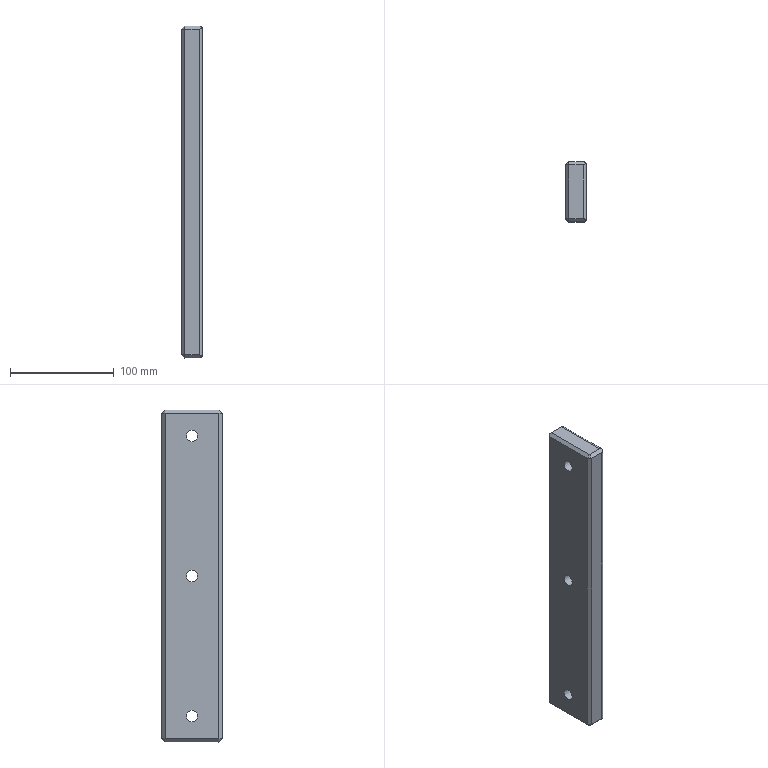Part | STEP file | lll_id1718_x_t | 1 solid | 31 faces | box 20 x 58 x 320 mm | volume 355635 mm3 | plane 21 | cylinder 10 | commonest cylinder face diameters 6 x4 11 x3 17 x3
STEP:
#1=CARTESIAN_POINT('',(2151.435,-651.5,-282.5));
#2=VERTEX_POINT('',#1);
#3=CARTESIAN_POINT('',(2151.435,-651.5,31.5));
#4=VERTEX_POINT('',#3);
#5=CARTESIAN_POINT('',(2151.435,-651.5,-55.5));
#6=DIRECTION('',(0.,-0.000000092,1.));
#7=VECTOR('',#6,1.);
#8=LINE('',#5,#7);
#9=EDGE_CURVE('',#2,#4,#8,.T.);
#10=ORIENTED_EDGE('',*,*,#9,.T.);
#11=CARTESIAN_POINT('',(2151.435,-599.5,31.5));
#12=VERTEX_POINT('',#11);
#13=CARTESIAN_POINT('',(2151.435,-644.5,31.5));
#14=DIRECTION('',(0.,1.,0.000000092));
#15=VECTOR('',#14,1.);
#16=LINE('',#13,#15);
#17=EDGE_CURVE('',#4,#12,#16,.T.);
#18=ORIENTED_EDGE('',*,*,#17,.T.);
#19=CARTESIAN_POINT('',(2151.435,-599.5,-282.5));
#20=VERTEX_POINT('',#19);
#21=CARTESIAN_POINT('',(2151.435,-599.5,69.5));
#22=DIRECTION('',(0.,0.000000092,-1.));
#23=VECTOR('',#22,1.);
#24=LINE('',#21,#23);
#25=EDGE_CURVE('',#12,#20,#24,.T.);
#26=ORIENTED_EDGE('',*,*,#25,.T.);
#27=CARTESIAN_POINT('',(2151.435,-596.5,-282.5));
#28=DIRECTION('',(0.,-1.,-0.000000092));
#29=VECTOR('',#28,1.);
#30=LINE('',#27,#29);
#31=EDGE_CURVE('',#20,#2,#30,.T.);
#32=ORIENTED_EDGE('',*,*,#31,.T.);
#33=EDGE_LOOP('',(#10,#18,#26,#32));
#34=FACE_BOUND('',#33,.T.);
#35=CARTESIAN_POINT('',(2151.435,-625.5,-266.));
#36=VERTEX_POINT('',#35);
#37=CARTESIAN_POINT('',(2151.435,-625.5,-260.5));
#38=DIRECTION('',(1.,0.,0.));
#39=DIRECTION('',(0.,0.,-1.));
#40=AXIS2_PLACEMENT_3D('',#37,#38,#39);
#41=CIRCLE('',#40,5.5);
#42=EDGE_CURVE('',#36,#36,#41,.T.);
#43=ORIENTED_EDGE('',*,*,#42,.T.);
#44=EDGE_LOOP('',(#43));
#45=FACE_BOUND('',#44,.T.);
#46=CARTESIAN_POINT('',(2151.435,-625.5,15.));
#47=VERTEX_POINT('',#46);
#48=CARTESIAN_POINT('',(2151.435,-625.5,9.5));
#49=DIRECTION('',(-1.,0.,0.));
#50=DIRECTION('',(0.,-0.000000184,1.));
#51=AXIS2_PLACEMENT_3D('',#48,#49,#50);
#52=CIRCLE('',#51,5.5);
#53=EDGE_CURVE('',#47,#47,#52,.T.);
#54=ORIENTED_EDGE('',*,*,#53,.F.);
#55=EDGE_LOOP('',(#54));
#56=FACE_BOUND('',#55,.T.);
#57=CARTESIAN_POINT('',(2151.435,-625.5,-131.));
#58=VERTEX_POINT('',#57);
#59=CARTESIAN_POINT('',(2151.435,-625.5,-125.5));
#60=DIRECTION('',(1.,0.,0.));
#61=DIRECTION('',(0.,0.,-1.));
#62=AXIS2_PLACEMENT_3D('',#59,#60,#61);
#63=CIRCLE('',#62,5.5);
#64=EDGE_CURVE('',#58,#58,#63,.T.);
#65=ORIENTED_EDGE('',*,*,#64,.T.);
#66=EDGE_LOOP('',(#65));
#67=FACE_BOUND('',#66,.T.);
#68=CARTESIAN_POINT('',(2151.435,-596.5,-55.5));
#69=DIRECTION('',(1.,0.,0.));
#70=DIRECTION('',(0.,-0.000000092,1.));
#71=AXIS2_PLACEMENT_3D('',#68,#69,#70);
#72=PLANE('',#71);
#73=ADVANCED_FACE('',(#34,#45,#56,#67),#72,.F.);
#74=CARTESIAN_POINT('',(2171.435,-625.5,-117.));
#75=VERTEX_POINT('',#74);
#76=CARTESIAN_POINT('',(2171.435,-625.5,-125.5));
#77=DIRECTION('',(-1.,0.,0.));
#78=DIRECTION('',(0.,0.,1.));
#79=AXIS2_PLACEMENT_3D('',#76,#77,#78);
#80=CIRCLE('',#79,8.5);
#81=EDGE_CURVE('',#75,#75,#80,.T.);
#82=ORIENTED_EDGE('',*,*,#81,.T.);
#83=EDGE_LOOP('',(#82));
#84=FACE_BOUND('',#83,.T.);
#85=CARTESIAN_POINT('',(2171.435,-599.5,31.5));
#86=VERTEX_POINT('',#85);
#87=CARTESIAN_POINT('',(2171.435,-599.5,-282.5));
#88=VERTEX_POINT('',#87);
#89=CARTESIAN_POINT('',(2171.435,-599.5,-55.5));
#90=DIRECTION('',(0.,0.000000092,-1.));
#91=VECTOR('',#90,1.);
#92=LINE('',#89,#91);
#93=EDGE_CURVE('',#86,#88,#92,.T.);
#94=ORIENTED_EDGE('',*,*,#93,.F.);
#95=CARTESIAN_POINT('',(2171.435,-651.5,31.5));
#96=VERTEX_POINT('',#95);
#97=CARTESIAN_POINT('',(2171.435,-644.5,31.5));
#98=DIRECTION('',(0.,-1.,-0.000000092));
#99=VECTOR('',#98,1.);
#100=LINE('',#97,#99);
#101=EDGE_CURVE('',#86,#96,#100,.T.);
#102=ORIENTED_EDGE('',*,*,#101,.T.);
#103=CARTESIAN_POINT('',(2171.435,-651.5,-282.5));
#104=VERTEX_POINT('',#103);
#105=CARTESIAN_POINT('',(2171.435,-651.5,-55.5));
#106=DIRECTION('',(0.,-0.000000092,1.));
#107=VECTOR('',#106,1.);
#108=LINE('',#105,#107);
#109=EDGE_CURVE('',#104,#96,#108,.T.);
#110=ORIENTED_EDGE('',*,*,#109,.F.);
#111=CARTESIAN_POINT('',(2171.435,-596.5,-282.5));
#112=DIRECTION('',(0.,-1.,-0.000000092));
#113=VECTOR('',#112,1.);
#114=LINE('',#111,#113);
#115=EDGE_CURVE('',#88,#104,#114,.T.);
#116=ORIENTED_EDGE('',*,*,#115,.F.);
#117=EDGE_LOOP('',(#94,#102,#110,#116));
#118=FACE_BOUND('',#117,.T.);
#119=CARTESIAN_POINT('',(2171.435,-625.5,-269.));
#120=VERTEX_POINT('',#119);
#121=CARTESIAN_POINT('',(2171.435,-625.5,-260.5));
#122=DIRECTION('',(-1.,0.,0.));
#123=DIRECTION('',(0.,0.,-1.));
#124=AXIS2_PLACEMENT_3D('',#121,#122,#123);
#125=CIRCLE('',#124,8.5);
#126=EDGE_CURVE('',#120,#120,#125,.T.);
#127=ORIENTED_EDGE('',*,*,#126,.T.);
#128=EDGE_LOOP('',(#127));
#129=FACE_BOUND('',#128,.T.);
#130=CARTESIAN_POINT('',(2171.435,-625.5,18.));
#131=VERTEX_POINT('',#130);
#132=CARTESIAN_POINT('',(2171.435,-625.5,9.5));
#133=DIRECTION('',(1.,0.,0.));
#134=DIRECTION('',(0.,-0.000000184,1.));
#135=AXIS2_PLACEMENT_3D('',#132,#133,#134);
#136=CIRCLE('',#135,8.5);
#137=EDGE_CURVE('',#131,#131,#136,.T.);
#138=ORIENTED_EDGE('',*,*,#137,.F.);
#139=EDGE_LOOP('',(#138));
#140=FACE_BOUND('',#139,.T.);
#141=CARTESIAN_POINT('',(2171.435,-596.5,-55.5));
#142=DIRECTION('',(1.,0.,0.));
#143=DIRECTION('',(0.,-0.000000092,1.));
#144=AXIS2_PLACEMENT_3D('',#141,#142,#143);
#145=PLANE('',#144);
#146=ADVANCED_FACE('',(#84,#118,#129,#140),#145,.T.);
#147=CARTESIAN_POINT('',(2154.435,-596.5,-282.5));
#148=VERTEX_POINT('',#147);
#149=CARTESIAN_POINT('',(2154.435,-596.5,31.5));
#150=VERTEX_POINT('',#149);
#151=CARTESIAN_POINT('',(2154.435,-596.5,69.5));
#152=DIRECTION('',(0.,-0.000000092,1.));
#153=VECTOR('',#152,1.);
#154=LINE('',#151,#153);
#155=EDGE_CURVE('',#148,#150,#154,.T.);
#156=ORIENTED_EDGE('',*,*,#155,.T.);
#157=CARTESIAN_POINT('',(2168.435,-596.5,31.5));
#158=VERTEX_POINT('',#157);
#159=CARTESIAN_POINT('',(2171.435,-596.5,31.5));
#160=DIRECTION('',(1.,0.,0.));
#161=VECTOR('',#160,1.);
#162=LINE('',#159,#161);
#163=EDGE_CURVE('',#150,#158,#162,.T.);
#164=ORIENTED_EDGE('',*,*,#163,.T.);
#165=CARTESIAN_POINT('',(2168.435,-596.5,-282.5));
#166=VERTEX_POINT('',#165);
#167=CARTESIAN_POINT('',(2168.435,-596.5,-55.5));
#168=DIRECTION('',(0.,-0.000000092,1.));
#169=VECTOR('',#168,1.);
#170=LINE('',#167,#169);
#171=EDGE_CURVE('',#166,#158,#170,.T.);
#172=ORIENTED_EDGE('',*,*,#171,.F.);
#173=CARTESIAN_POINT('',(2171.435,-596.5,-282.5));
#174=DIRECTION('',(-1.,0.,0.));
#175=VECTOR('',#174,1.);
#176=LINE('',#173,#175);
#177=EDGE_CURVE('',#166,#148,#176,.T.);
#178=ORIENTED_EDGE('',*,*,#177,.T.);
#179=EDGE_LOOP('',(#156,#164,#172,#178));
#180=FACE_OUTER_BOUND('',#179,.T.);
#181=CARTESIAN_POINT('',(2171.435,-596.5,69.5));
#182=DIRECTION('',(0.,-1.,-0.000000092));
#183=DIRECTION('',(0.,0.000000092,-1.));
#184=AXIS2_PLACEMENT_3D('',#181,#182,#183);
#185=PLANE('',#184);
#186=ADVANCED_FACE('',(#180),#185,.F.);
#187=CARTESIAN_POINT('',(2168.435,-654.5,31.5));
#188=VERTEX_POINT('',#187);
#189=CARTESIAN_POINT('',(2168.435,-654.5,-282.5));
#190=VERTEX_POINT('',#189);
#191=CARTESIAN_POINT('',(2168.435,-654.5,69.5));
#192=DIRECTION('',(0.,0.000000092,-1.));
#193=VECTOR('',#192,1.);
#194=LINE('',#191,#193);
#195=EDGE_CURVE('',#188,#190,#194,.T.);
#196=ORIENTED_EDGE('',*,*,#195,.F.);
#197=CARTESIAN_POINT('',(2154.435,-654.5,31.5));
#198=VERTEX_POINT('',#197);
#199=CARTESIAN_POINT('',(2171.435,-654.5,31.5));
#200=DIRECTION('',(-1.,0.,0.));
#201=VECTOR('',#200,1.);
#202=LINE('',#199,#201);
#203=EDGE_CURVE('',#188,#198,#202,.T.);
#204=ORIENTED_EDGE('',*,*,#203,.T.);
#205=CARTESIAN_POINT('',(2154.435,-654.5,-282.5));
#206=VERTEX_POINT('',#205);
#207=CARTESIAN_POINT('',(2154.435,-654.5,-55.5));
#208=DIRECTION('',(0.,0.000000092,-1.));
#209=VECTOR('',#208,1.);
#210=LINE('',#207,#209);
#211=EDGE_CURVE('',#198,#206,#210,.T.);
#212=ORIENTED_EDGE('',*,*,#211,.T.);
#213=CARTESIAN_POINT('',(2171.435,-654.5,-282.5));
#214=DIRECTION('',(1.,0.,0.));
#215=VECTOR('',#214,1.);
#216=LINE('',#213,#215);
#217=EDGE_CURVE('',#206,#190,#216,.T.);
#218=ORIENTED_EDGE('',*,*,#217,.T.);
#219=EDGE_LOOP('',(#196,#204,#212,#218));
#220=FACE_OUTER_BOUND('',#219,.T.);
#221=CARTESIAN_POINT('',(2171.435,-654.5,-55.5));
#222=DIRECTION('',(0.,1.,0.000000092));
#223=DIRECTION('',(0.,-0.000000092,1.));
#224=AXIS2_PLACEMENT_3D('',#221,#222,#223);
#225=PLANE('',#224);
#226=ADVANCED_FACE('',(#220),#225,.F.);
#227=ORIENTED_EDGE('',*,*,#171,.T.);
#228=CARTESIAN_POINT('',(2171.033,-598.,33.));
#229=VERTEX_POINT('',#228);
#230=CARTESIAN_POINT('',(2168.435,-599.5,34.5));
#231=DIRECTION('',(0.,-0.7071,-0.7071));
#232=DIRECTION('',(0.,-0.7071,0.7071));
#233=AXIS2_PLACEMENT_3D('',#230,#231,#232);
#234=ELLIPSE('',#233,4.243,3.);
#235=EDGE_CURVE('',#158,#229,#234,.T.);
#236=ORIENTED_EDGE('',*,*,#235,.T.);
#237=CARTESIAN_POINT('',(2168.435,-599.5,31.5));
#238=DIRECTION('',(0.,0.7071,-0.7071));
#239=DIRECTION('',(0.,0.7071,0.7071));
#240=AXIS2_PLACEMENT_3D('',#237,#238,#239);
#241=ELLIPSE('',#240,4.243,3.);
#242=EDGE_CURVE('',#229,#86,#241,.T.);
#243=ORIENTED_EDGE('',*,*,#242,.T.);
#244=ORIENTED_EDGE('',*,*,#93,.T.);
#245=CARTESIAN_POINT('',(2171.033,-598.,-284.));
#246=VERTEX_POINT('',#245);
#247=CARTESIAN_POINT('',(2168.435,-599.5,-282.5));
#248=DIRECTION('',(0.,-0.7071,-0.7071));
#249=DIRECTION('',(0.,0.7071,-0.7071));
#250=AXIS2_PLACEMENT_3D('',#247,#248,#249);
#251=ELLIPSE('',#250,4.243,3.);
#252=EDGE_CURVE('',#246,#88,#251,.T.);
#253=ORIENTED_EDGE('',*,*,#252,.F.);
#254=CARTESIAN_POINT('',(2168.435,-599.5,-285.5));
#255=DIRECTION('',(0.,-0.7071,0.7071));
#256=DIRECTION('',(0.,0.7071,0.7071));
#257=AXIS2_PLACEMENT_3D('',#254,#255,#256);
#258=ELLIPSE('',#257,4.243,3.);
#259=EDGE_CURVE('',#246,#166,#258,.T.);
#260=ORIENTED_EDGE('',*,*,#259,.T.);
#261=EDGE_LOOP('',(#227,#236,#243,#244,#253,#260));
#262=FACE_OUTER_BOUND('',#261,.T.);
#263=CARTESIAN_POINT('',(2168.435,-599.5,69.5));
#264=DIRECTION('',(0.,-0.000000092,1.));
#265=DIRECTION('',(1.,0.,0.));
#266=AXIS2_PLACEMENT_3D('',#263,#264,#265);
#267=CYLINDRICAL_SURFACE('',#266,3.);
#268=ADVANCED_FACE('',(#262),#267,.T.);
#269=ORIENTED_EDGE('',*,*,#109,.T.);
#270=CARTESIAN_POINT('',(2171.033,-653.,33.));
#271=VERTEX_POINT('',#270);
#272=CARTESIAN_POINT('',(2168.435,-651.5,31.5));
#273=DIRECTION('',(0.,-0.7071,-0.7071));
#274=DIRECTION('',(0.,0.7071,-0.7071));
#275=AXIS2_PLACEMENT_3D('',#272,#273,#274);
#276=ELLIPSE('',#275,4.243,3.);
#277=EDGE_CURVE('',#96,#271,#276,.T.);
#278=ORIENTED_EDGE('',*,*,#277,.T.);
#279=CARTESIAN_POINT('',(2168.435,-651.5,34.5));
#280=DIRECTION('',(0.,0.7071,-0.7071));
#281=DIRECTION('',(0.,-0.7071,-0.7071));
#282=AXIS2_PLACEMENT_3D('',#279,#280,#281);
#283=ELLIPSE('',#282,4.243,3.);
#284=EDGE_CURVE('',#271,#188,#283,.T.);
#285=ORIENTED_EDGE('',*,*,#284,.T.);
#286=ORIENTED_EDGE('',*,*,#195,.T.);
#287=CARTESIAN_POINT('',(2171.033,-653.,-284.));
#288=VERTEX_POINT('',#287);
#289=CARTESIAN_POINT('',(2168.435,-651.5,-285.5));
#290=DIRECTION('',(0.,0.7071,0.7071));
#291=DIRECTION('',(0.,0.7071,-0.7071));
#292=AXIS2_PLACEMENT_3D('',#289,#290,#291);
#293=ELLIPSE('',#292,4.243,3.);
#294=EDGE_CURVE('',#190,#288,#293,.T.);
#295=ORIENTED_EDGE('',*,*,#294,.T.);
#296=CARTESIAN_POINT('',(2168.435,-651.5,-282.5));
#297=DIRECTION('',(0.,0.7071,-0.7071));
#298=DIRECTION('',(0.,0.7071,0.7071));
#299=AXIS2_PLACEMENT_3D('',#296,#297,#298);
#300=ELLIPSE('',#299,4.243,3.);
#301=EDGE_CURVE('',#104,#288,#300,.T.);
#302=ORIENTED_EDGE('',*,*,#301,.F.);
#303=EDGE_LOOP('',(#269,#278,#285,#286,#295,#302));
#304=FACE_OUTER_BOUND('',#303,.T.);
#305=CARTESIAN_POINT('',(2168.435,-651.5,-55.5));
#306=DIRECTION('',(0.,0.000000092,-1.));
#307=DIRECTION('',(-1.,0.,0.));
#308=AXIS2_PLACEMENT_3D('',#305,#306,#307);
#309=CYLINDRICAL_SURFACE('',#308,3.);
#310=ADVANCED_FACE('',(#304),#309,.T.);
#311=ORIENTED_EDGE('',*,*,#211,.F.);
#312=CARTESIAN_POINT('',(2154.435,-654.5,31.5));
#313=DIRECTION('',(-0.7071,0.7071,0.000000065));
#314=VECTOR('',#313,1.);
#315=LINE('',#312,#314);
#316=EDGE_CURVE('',#198,#4,#315,.T.);
#317=ORIENTED_EDGE('',*,*,#316,.T.);
#318=ORIENTED_EDGE('',*,*,#9,.F.);
#319=CARTESIAN_POINT('',(2154.435,-654.5,-282.5));
#320=DIRECTION('',(-0.7071,0.7071,0.000000065));
#321=VECTOR('',#320,1.);
#322=LINE('',#319,#321);
#323=EDGE_CURVE('',#206,#2,#322,.T.);
#324=ORIENTED_EDGE('',*,*,#323,.F.);
#325=EDGE_LOOP('',(#311,#317,#318,#324));
#326=FACE_OUTER_BOUND('',#325,.T.);
#327=CARTESIAN_POINT('',(2154.435,-654.5,-55.5));
#328=DIRECTION('',(0.7071,0.7071,0.000000065));
#329=DIRECTION('',(0.7071,-0.7071,-0.000000065));
#330=AXIS2_PLACEMENT_3D('',#327,#328,#329);
#331=PLANE('',#330);
#332=ADVANCED_FACE('',(#326),#331,.F.);
#333=ORIENTED_EDGE('',*,*,#25,.F.);
#334=CARTESIAN_POINT('',(2154.435,-596.5,31.5));
#335=DIRECTION('',(0.7071,0.7071,0.000000065));
#336=VECTOR('',#335,1.);
#337=LINE('',#334,#336);
#338=EDGE_CURVE('',#12,#150,#337,.T.);
#339=ORIENTED_EDGE('',*,*,#338,.T.);
#340=ORIENTED_EDGE('',*,*,#155,.F.);
#341=CARTESIAN_POINT('',(2154.435,-596.5,-282.5));
#342=DIRECTION('',(0.7071,0.7071,0.000000065));
#343=VECTOR('',#342,1.);
#344=LINE('',#341,#343);
#345=EDGE_CURVE('',#20,#148,#344,.T.);
#346=ORIENTED_EDGE('',*,*,#345,.F.);
#347=EDGE_LOOP('',(#333,#339,#340,#346));
#348=FACE_OUTER_BOUND('',#347,.T.);
#349=CARTESIAN_POINT('',(2154.435,-596.5,69.5));
#350=DIRECTION('',(0.7071,-0.7071,-0.000000065));
#351=DIRECTION('',(-0.7071,-0.7071,-0.000000065));
#352=AXIS2_PLACEMENT_3D('',#349,#350,#351);
#353=PLANE('',#352);
#354=ADVANCED_FACE('',(#348),#353,.F.);
#355=CARTESIAN_POINT('',(2168.435,-651.5,-285.5));
#356=VERTEX_POINT('',#355);
#357=CARTESIAN_POINT('',(2168.435,-599.5,-285.5));
#358=VERTEX_POINT('',#357);
#359=CARTESIAN_POINT('',(2168.435,-644.5,-285.5));
#360=DIRECTION('',(0.,1.,0.000000092));
#361=VECTOR('',#360,1.);
#362=LINE('',#359,#361);
#363=EDGE_CURVE('',#356,#358,#362,.T.);
#364=ORIENTED_EDGE('',*,*,#363,.F.);
#365=CARTESIAN_POINT('',(2154.435,-651.5,-285.5));
#366=VERTEX_POINT('',#365);
#367=CARTESIAN_POINT('',(2171.435,-651.5,-285.5));
#368=DIRECTION('',(-1.,0.,0.));
#369=VECTOR('',#368,1.);
#370=LINE('',#367,#369);
#371=EDGE_CURVE('',#356,#366,#370,.T.);
#372=ORIENTED_EDGE('',*,*,#371,.T.);
#373=CARTESIAN_POINT('',(2154.435,-599.5,-285.5));
#374=VERTEX_POINT('',#373);
#375=CARTESIAN_POINT('',(2154.435,-596.5,-285.5));
#376=DIRECTION('',(0.,1.,0.000000092));
#377=VECTOR('',#376,1.);
#378=LINE('',#375,#377);
#379=EDGE_CURVE('',#366,#374,#378,.T.);
#380=ORIENTED_EDGE('',*,*,#379,.T.);
#381=CARTESIAN_POINT('',(2171.435,-599.5,-285.5));
#382=DIRECTION('',(1.,0.,0.));
#383=VECTOR('',#382,1.);
#384=LINE('',#381,#383);
#385=EDGE_CURVE('',#374,#358,#384,.T.);
#386=ORIENTED_EDGE('',*,*,#385,.T.);
#387=EDGE_LOOP('',(#364,#372,#380,#386));
#388=FACE_OUTER_BOUND('',#387,.T.);
#389=CARTESIAN_POINT('',(2171.435,-596.5,-285.5));
#390=DIRECTION('',(0.,-0.000000092,1.));
#391=DIRECTION('',(-1.,0.,0.));
#392=AXIS2_PLACEMENT_3D('',#389,#390,#391);
#393=PLANE('',#392);
#394=ADVANCED_FACE('',(#388),#393,.F.);
#395=CARTESIAN_POINT('',(2159.435,-625.5,-266.));
#396=VERTEX_POINT('',#395);
#397=CARTESIAN_POINT('',(2159.435,-625.5,-260.5));
#398=DIRECTION('',(-1.,0.,0.));
#399=DIRECTION('',(0.,0.000000092,-1.));
#400=AXIS2_PLACEMENT_3D('',#397,#398,#399);
#401=CIRCLE('',#400,5.5);
#402=EDGE_CURVE('',#396,#396,#401,.T.);
#403=ORIENTED_EDGE('',*,*,#402,.F.);
#404=EDGE_LOOP('',(#403));
#405=FACE_BOUND('',#404,.T.);
#406=ORIENTED_EDGE('',*,*,#42,.F.);
#407=EDGE_LOOP('',(#406));
#408=FACE_BOUND('',#407,.T.);
#409=CARTESIAN_POINT('',(2111.435,-625.5,-260.5));
#410=DIRECTION('',(-1.,0.,0.));
#411=DIRECTION('',(0.,0.000000092,-1.));
#412=AXIS2_PLACEMENT_3D('',#409,#410,#411);
#413=CYLINDRICAL_SURFACE('',#412,5.5);
#414=ADVANCED_FACE('',(#405,#408),#413,.F.);
#415=ORIENTED_EDGE('',*,*,#402,.T.);
#416=EDGE_LOOP('',(#415));
#417=FACE_BOUND('',#416,.T.);
#418=CARTESIAN_POINT('',(2159.435,-625.5,-269.));
#419=VERTEX_POINT('',#418);
#420=CARTESIAN_POINT('',(2159.435,-625.5,-260.5));
#421=DIRECTION('',(-1.,0.,0.));
#422=DIRECTION('',(0.,0.000000092,-1.));
#423=AXIS2_PLACEMENT_3D('',#420,#421,#422);
#424=CIRCLE('',#423,8.5);
#425=EDGE_CURVE('',#419,#419,#424,.T.);
#426=ORIENTED_EDGE('',*,*,#425,.F.);
#427=EDGE_LOOP('',(#426));
#428=FACE_BOUND('',#427,.T.);
#429=CARTESIAN_POINT('',(2159.435,-625.5,-260.5));
#430=DIRECTION('',(-1.,0.,0.));
#431=DIRECTION('',(0.,0.000000092,-1.));
#432=AXIS2_PLACEMENT_3D('',#429,#430,#431);
#433=PLANE('',#432);
#434=ADVANCED_FACE('',(#417,#428),#433,.F.);
#435=ORIENTED_EDGE('',*,*,#425,.T.);
#436=EDGE_LOOP('',(#435));
#437=FACE_BOUND('',#436,.T.);
#438=ORIENTED_EDGE('',*,*,#126,.F.);
#439=EDGE_LOOP('',(#438));
#440=FACE_BOUND('',#439,.T.);
#441=CARTESIAN_POINT('',(2171.435,-625.5,-260.5));
#442=DIRECTION('',(-1.,0.,0.));
#443=DIRECTION('',(0.,0.000000092,-1.));
#444=AXIS2_PLACEMENT_3D('',#441,#442,#443);
#445=CYLINDRICAL_SURFACE('',#444,8.5);
#446=ADVANCED_FACE('',(#437,#440),#445,.F.);
#447=ORIENTED_EDGE('',*,*,#252,.T.);
#448=ORIENTED_EDGE('',*,*,#115,.T.);
#449=ORIENTED_EDGE('',*,*,#301,.T.);
#450=CARTESIAN_POINT('',(2168.435,-654.5,-282.5));
#451=DIRECTION('',(0.,0.7071,0.7071));
#452=DIRECTION('',(0.,0.7071,-0.7071));
#453=AXIS2_PLACEMENT_3D('',#450,#451,#452);
#454=ELLIPSE('',#453,4.243,3.);
#455=EDGE_CURVE('',#288,#356,#454,.T.);
#456=ORIENTED_EDGE('',*,*,#455,.T.);
#457=ORIENTED_EDGE('',*,*,#363,.T.);
#458=CARTESIAN_POINT('',(2168.435,-596.5,-282.5));
#459=DIRECTION('',(0.,-0.7071,0.7071));
#460=DIRECTION('',(0.,0.7071,0.7071));
#461=AXIS2_PLACEMENT_3D('',#458,#459,#460);
#462=ELLIPSE('',#461,4.243,3.);
#463=EDGE_CURVE('',#358,#246,#462,.T.);
#464=ORIENTED_EDGE('',*,*,#463,.T.);
#465=EDGE_LOOP('',(#447,#448,#449,#456,#457,#464));
#466=FACE_OUTER_BOUND('',#465,.T.);
#467=CARTESIAN_POINT('',(2168.435,-596.5,-282.5));
#468=DIRECTION('',(0.,1.,0.000000092));
#469=DIRECTION('',(0.,-0.000000092,1.));
#470=AXIS2_PLACEMENT_3D('',#467,#468,#469);
#471=CYLINDRICAL_SURFACE('',#470,3.);
#472=ADVANCED_FACE('',(#466),#471,.T.);
#473=ORIENTED_EDGE('',*,*,#455,.F.);
#474=ORIENTED_EDGE('',*,*,#294,.F.);
#475=ORIENTED_EDGE('',*,*,#217,.F.);
#476=CARTESIAN_POINT('',(2154.435,-651.5,-285.5));
#477=DIRECTION('',(0.,-0.7071,0.7071));
#478=VECTOR('',#477,1.);
#479=LINE('',#476,#478);
#480=EDGE_CURVE('',#366,#206,#479,.T.);
#481=ORIENTED_EDGE('',*,*,#480,.F.);
#482=ORIENTED_EDGE('',*,*,#371,.F.);
#483=EDGE_LOOP('',(#473,#474,#475,#481,#482));
#484=FACE_OUTER_BOUND('',#483,.T.);
#485=CARTESIAN_POINT('',(2171.435,-654.5,-282.5));
#486=DIRECTION('',(0.,0.7071,0.7071));
#487=DIRECTION('',(0.,0.7071,-0.7071));
#488=AXIS2_PLACEMENT_3D('',#485,#486,#487);
#489=PLANE('',#488);
#490=ADVANCED_FACE('',(#484),#489,.F.);
#491=ORIENTED_EDGE('',*,*,#323,.T.);
#492=CARTESIAN_POINT('',(2154.435,-651.5,-285.5));
#493=DIRECTION('',(-0.7071,-0.000000065,0.7071));
#494=VECTOR('',#493,1.);
#495=LINE('',#492,#494);
#496=EDGE_CURVE('',#366,#2,#495,.T.);
#497=ORIENTED_EDGE('',*,*,#496,.F.);
#498=ORIENTED_EDGE('',*,*,#480,.T.);
#499=EDGE_LOOP('',(#491,#497,#498));
#500=FACE_OUTER_BOUND('',#499,.T.);
#501=CARTESIAN_POINT('',(2154.435,-651.5,-285.5));
#502=DIRECTION('',(-0.5774,-0.5774,-0.5774));
#503=DIRECTION('',(-0.7071,-0.000000065,0.7071));
#504=AXIS2_PLACEMENT_3D('',#501,#502,#503);
#505=PLANE('',#504);
#506=ADVANCED_FACE('',(#500),#505,.T.);
#507=ORIENTED_EDGE('',*,*,#496,.T.);
#508=ORIENTED_EDGE('',*,*,#31,.F.);
#509=CARTESIAN_POINT('',(2154.435,-599.5,-285.5));
#510=DIRECTION('',(-0.7071,-0.000000065,0.7071));
#511=VECTOR('',#510,1.);
#512=LINE('',#509,#511);
#513=EDGE_CURVE('',#374,#20,#512,.T.);
#514=ORIENTED_EDGE('',*,*,#513,.F.);
#515=ORIENTED_EDGE('',*,*,#379,.F.);
#516=EDGE_LOOP('',(#507,#508,#514,#515));
#517=FACE_OUTER_BOUND('',#516,.T.);
#518=CARTESIAN_POINT('',(2154.435,-596.5,-285.5));
#519=DIRECTION('',(0.7071,-0.000000065,0.7071));
#520=DIRECTION('',(0.7071,0.000000065,-0.7071));
#521=AXIS2_PLACEMENT_3D('',#518,#519,#520);
#522=PLANE('',#521);
#523=ADVANCED_FACE('',(#517),#522,.F.);
#524=ORIENTED_EDGE('',*,*,#345,.T.);
#525=CARTESIAN_POINT('',(2154.435,-599.5,-285.5));
#526=DIRECTION('',(0.,0.7071,0.7071));
#527=VECTOR('',#526,1.);
#528=LINE('',#525,#527);
#529=EDGE_CURVE('',#374,#148,#528,.T.);
#530=ORIENTED_EDGE('',*,*,#529,.F.);
#531=ORIENTED_EDGE('',*,*,#513,.T.);
#532=EDGE_LOOP('',(#524,#530,#531));
#533=FACE_OUTER_BOUND('',#532,.T.);
#534=CARTESIAN_POINT('',(2154.435,-599.5,-285.5));
#535=DIRECTION('',(-0.5774,0.5774,-0.5774));
#536=DIRECTION('',(-0.7071,-0.000000065,0.7071));
#537=AXIS2_PLACEMENT_3D('',#534,#535,#536);
#538=PLANE('',#537);
#539=ADVANCED_FACE('',(#533),#538,.T.);
#540=ORIENTED_EDGE('',*,*,#259,.F.);
#541=ORIENTED_EDGE('',*,*,#463,.F.);
#542=ORIENTED_EDGE('',*,*,#385,.F.);
#543=ORIENTED_EDGE('',*,*,#529,.T.);
#544=ORIENTED_EDGE('',*,*,#177,.F.);
#545=EDGE_LOOP('',(#540,#541,#542,#543,#544));
#546=FACE_OUTER_BOUND('',#545,.T.);
#547=CARTESIAN_POINT('',(2171.435,-599.5,-285.5));
#548=DIRECTION('',(0.,-0.7071,0.7071));
#549=DIRECTION('',(0.,0.7071,0.7071));
#550=AXIS2_PLACEMENT_3D('',#547,#548,#549);
#551=PLANE('',#550);
#552=ADVANCED_FACE('',(#546),#551,.F.);
#553=CARTESIAN_POINT('',(2154.435,-599.5,34.5));
#554=VERTEX_POINT('',#553);
#555=CARTESIAN_POINT('',(2154.435,-651.5,34.5));
#556=VERTEX_POINT('',#555);
#557=CARTESIAN_POINT('',(2154.435,-644.5,34.5));
#558=DIRECTION('',(0.,-1.,-0.000000092));
#559=VECTOR('',#558,1.);
#560=LINE('',#557,#559);
#561=EDGE_CURVE('',#554,#556,#560,.T.);
#562=ORIENTED_EDGE('',*,*,#561,.T.);
#563=CARTESIAN_POINT('',(2168.435,-651.5,34.5));
#564=VERTEX_POINT('',#563);
#565=CARTESIAN_POINT('',(2171.435,-651.5,34.5));
#566=DIRECTION('',(1.,0.,0.));
#567=VECTOR('',#566,1.);
#568=LINE('',#565,#567);
#569=EDGE_CURVE('',#556,#564,#568,.T.);
#570=ORIENTED_EDGE('',*,*,#569,.T.);
#571=CARTESIAN_POINT('',(2168.435,-599.5,34.5));
#572=VERTEX_POINT('',#571);
#573=CARTESIAN_POINT('',(2168.435,-644.5,34.5));
#574=DIRECTION('',(0.,1.,0.000000092));
#575=VECTOR('',#574,1.);
#576=LINE('',#573,#575);
#577=EDGE_CURVE('',#564,#572,#576,.T.);
#578=ORIENTED_EDGE('',*,*,#577,.T.);
#579=CARTESIAN_POINT('',(2171.435,-599.5,34.5));
#580=DIRECTION('',(-1.,0.,0.));
#581=VECTOR('',#580,1.);
#582=LINE('',#579,#581);
#583=EDGE_CURVE('',#572,#554,#582,.T.);
#584=ORIENTED_EDGE('',*,*,#583,.T.);
#585=EDGE_LOOP('',(#562,#570,#578,#584));
#586=FACE_OUTER_BOUND('',#585,.T.);
#587=CARTESIAN_POINT('',(2171.435,-644.5,34.5));
#588=DIRECTION('',(0.,0.000000092,-1.));
#589=DIRECTION('',(1.,0.,0.));
#590=AXIS2_PLACEMENT_3D('',#587,#588,#589);
#591=PLANE('',#590);
#592=ADVANCED_FACE('',(#586),#591,.F.);
#593=CARTESIAN_POINT('',(2154.435,-651.5,34.5));
#594=DIRECTION('',(0.7071,-0.000000065,0.7071));
#595=VECTOR('',#594,1.);
#596=LINE('',#593,#595);
#597=EDGE_CURVE('',#4,#556,#596,.T.);
#598=ORIENTED_EDGE('',*,*,#597,.T.);
#599=ORIENTED_EDGE('',*,*,#561,.F.);
#600=CARTESIAN_POINT('',(2152.935,-599.5,33.));
#601=DIRECTION('',(0.7071,-0.000000065,0.7071));
#602=VECTOR('',#601,1.);
#603=LINE('',#600,#602);
#604=EDGE_CURVE('',#12,#554,#603,.T.);
#605=ORIENTED_EDGE('',*,*,#604,.F.);
#606=ORIENTED_EDGE('',*,*,#17,.F.);
#607=EDGE_LOOP('',(#598,#599,#605,#606));
#608=FACE_OUTER_BOUND('',#607,.T.);
#609=CARTESIAN_POINT('',(2154.435,-644.5,34.5));
#610=DIRECTION('',(0.7071,0.000000065,-0.7071));
#611=DIRECTION('',(-0.7071,0.000000065,-0.7071));
#612=AXIS2_PLACEMENT_3D('',#609,#610,#611);
#613=PLANE('',#612);
#614=ADVANCED_FACE('',(#608),#613,.F.);
#615=CARTESIAN_POINT('',(2168.435,-596.5,31.5));
#616=DIRECTION('',(0.,-0.7071,-0.7071));
#617=DIRECTION('',(0.,0.7071,-0.7071));
#618=AXIS2_PLACEMENT_3D('',#615,#616,#617);
#619=ELLIPSE('',#618,4.243,3.);
#620=EDGE_CURVE('',#229,#572,#619,.T.);
#621=ORIENTED_EDGE('',*,*,#620,.F.);
#622=ORIENTED_EDGE('',*,*,#235,.F.);
#623=ORIENTED_EDGE('',*,*,#163,.F.);
#624=CARTESIAN_POINT('',(2154.435,-596.5,31.5));
#625=DIRECTION('',(0.,0.7071,-0.7071));
#626=VECTOR('',#625,1.);
#627=LINE('',#624,#626);
#628=EDGE_CURVE('',#554,#150,#627,.T.);
#629=ORIENTED_EDGE('',*,*,#628,.F.);
#630=ORIENTED_EDGE('',*,*,#583,.F.);
#631=EDGE_LOOP('',(#621,#622,#623,#629,#630));
#632=FACE_OUTER_BOUND('',#631,.T.);
#633=CARTESIAN_POINT('',(2171.435,-596.5,31.5));
#634=DIRECTION('',(0.,-0.7071,-0.7071));
#635=DIRECTION('',(0.,-0.7071,0.7071));
#636=AXIS2_PLACEMENT_3D('',#633,#634,#635);
#637=PLANE('',#636);
#638=ADVANCED_FACE('',(#632),#637,.F.);
#639=CARTESIAN_POINT('',(2154.435,-654.5,31.5));
#640=DIRECTION('',(0.,0.7071,0.7071));
#641=VECTOR('',#640,1.);
#642=LINE('',#639,#641);
#643=EDGE_CURVE('',#198,#556,#642,.T.);
#644=ORIENTED_EDGE('',*,*,#643,.F.);
#645=ORIENTED_EDGE('',*,*,#203,.F.);
#646=ORIENTED_EDGE('',*,*,#284,.F.);
#647=CARTESIAN_POINT('',(2168.435,-654.5,31.5));
#648=DIRECTION('',(0.,0.7071,-0.7071));
#649=DIRECTION('',(0.,0.7071,0.7071));
#650=AXIS2_PLACEMENT_3D('',#647,#648,#649);
#651=ELLIPSE('',#650,4.243,3.);
#652=EDGE_CURVE('',#564,#271,#651,.T.);
#653=ORIENTED_EDGE('',*,*,#652,.F.);
#654=ORIENTED_EDGE('',*,*,#569,.F.);
#655=EDGE_LOOP('',(#644,#645,#646,#653,#654));
#656=FACE_OUTER_BOUND('',#655,.T.);
#657=CARTESIAN_POINT('',(2171.435,-651.5,34.5));
#658=DIRECTION('',(0.,0.7071,-0.7071));
#659=DIRECTION('',(0.,-0.7071,-0.7071));
#660=AXIS2_PLACEMENT_3D('',#657,#658,#659);
#661=PLANE('',#660);
#662=ADVANCED_FACE('',(#656),#661,.F.);
#663=ORIENTED_EDGE('',*,*,#577,.F.);
#664=ORIENTED_EDGE('',*,*,#652,.T.);
#665=ORIENTED_EDGE('',*,*,#277,.F.);
#666=ORIENTED_EDGE('',*,*,#101,.F.);
#667=ORIENTED_EDGE('',*,*,#242,.F.);
#668=ORIENTED_EDGE('',*,*,#620,.T.);
#669=EDGE_LOOP('',(#663,#664,#665,#666,#667,#668));
#670=FACE_OUTER_BOUND('',#669,.T.);
#671=CARTESIAN_POINT('',(2168.435,-644.5,31.5));
#672=DIRECTION('',(0.,1.,0.000000092));
#673=DIRECTION('',(0.,0.000000092,-1.));
#674=AXIS2_PLACEMENT_3D('',#671,#672,#673);
#675=CYLINDRICAL_SURFACE('',#674,3.);
#676=ADVANCED_FACE('',(#670),#675,.T.);
#677=ORIENTED_EDGE('',*,*,#597,.F.);
#678=ORIENTED_EDGE('',*,*,#316,.F.);
#679=ORIENTED_EDGE('',*,*,#643,.T.);
#680=EDGE_LOOP('',(#677,#678,#679));
#681=FACE_OUTER_BOUND('',#680,.T.);
#682=CARTESIAN_POINT('',(2154.435,-654.5,31.5));
#683=DIRECTION('',(-0.5774,-0.5774,0.5774));
#684=DIRECTION('',(0.7071,-0.000000065,0.7071));
#685=AXIS2_PLACEMENT_3D('',#682,#683,#684);
#686=PLANE('',#685);
#687=ADVANCED_FACE('',(#681),#686,.T.);
#688=ORIENTED_EDGE('',*,*,#628,.T.);
#689=ORIENTED_EDGE('',*,*,#338,.F.);
#690=ORIENTED_EDGE('',*,*,#604,.T.);
#691=EDGE_LOOP('',(#688,#689,#690));
#692=FACE_OUTER_BOUND('',#691,.T.);
#693=CARTESIAN_POINT('',(2154.435,-596.5,31.5));
#694=DIRECTION('',(-0.5774,0.5774,0.5774));
#695=DIRECTION('',(0.7071,-0.000000065,0.7071));
#696=AXIS2_PLACEMENT_3D('',#693,#694,#695);
#697=PLANE('',#696);
#698=ADVANCED_FACE('',(#692),#697,.T.);
#699=CARTESIAN_POINT('',(2159.435,-625.5,18.));
#700=VERTEX_POINT('',#699);
#701=CARTESIAN_POINT('',(2159.435,-625.5,9.5));
#702=DIRECTION('',(1.,0.,0.));
#703=DIRECTION('',(0.,-0.000000092,1.));
#704=AXIS2_PLACEMENT_3D('',#701,#702,#703);
#705=CIRCLE('',#704,8.5);
#706=EDGE_CURVE('',#700,#700,#705,.T.);
#707=ORIENTED_EDGE('',*,*,#706,.F.);
#708=EDGE_LOOP('',(#707));
#709=FACE_BOUND('',#708,.T.);
#710=ORIENTED_EDGE('',*,*,#137,.T.);
#711=EDGE_LOOP('',(#710));
#712=FACE_BOUND('',#711,.T.);
#713=CARTESIAN_POINT('',(2171.435,-625.5,9.5));
#714=DIRECTION('',(-1.,0.,0.));
#715=DIRECTION('',(0.,-0.000000092,1.));
#716=AXIS2_PLACEMENT_3D('',#713,#714,#715);
#717=CYLINDRICAL_SURFACE('',#716,8.5);
#718=ADVANCED_FACE('',(#709,#712),#717,.F.);
#719=CARTESIAN_POINT('',(2159.435,-625.5,15.));
#720=VERTEX_POINT('',#719);
#721=CARTESIAN_POINT('',(2159.435,-625.5,9.5));
#722=DIRECTION('',(1.,0.,0.));
#723=DIRECTION('',(0.,-0.000000092,1.));
#724=AXIS2_PLACEMENT_3D('',#721,#722,#723);
#725=CIRCLE('',#724,5.5);
#726=EDGE_CURVE('',#720,#720,#725,.T.);
#727=ORIENTED_EDGE('',*,*,#726,.T.);
#728=EDGE_LOOP('',(#727));
#729=FACE_BOUND('',#728,.T.);
#730=ORIENTED_EDGE('',*,*,#53,.T.);
#731=EDGE_LOOP('',(#730));
#732=FACE_BOUND('',#731,.T.);
#733=CARTESIAN_POINT('',(2111.435,-625.5,9.5));
#734=DIRECTION('',(-1.,0.,0.));
#735=DIRECTION('',(0.,-0.000000092,1.));
#736=AXIS2_PLACEMENT_3D('',#733,#734,#735);
#737=CYLINDRICAL_SURFACE('',#736,5.5);
#738=ADVANCED_FACE('',(#729,#732),#737,.F.);
#739=ORIENTED_EDGE('',*,*,#726,.F.);
#740=EDGE_LOOP('',(#739));
#741=FACE_BOUND('',#740,.T.);
#742=ORIENTED_EDGE('',*,*,#706,.T.);
#743=EDGE_LOOP('',(#742));
#744=FACE_BOUND('',#743,.T.);
#745=CARTESIAN_POINT('',(2159.435,-625.5,9.5));
#746=DIRECTION('',(-1.,0.,0.));
#747=DIRECTION('',(0.,-0.000000092,1.));
#748=AXIS2_PLACEMENT_3D('',#745,#746,#747);
#749=PLANE('',#748);
#750=ADVANCED_FACE('',(#741,#744),#749,.F.);
#751=ORIENTED_EDGE('',*,*,#81,.F.);
#752=EDGE_LOOP('',(#751));
#753=FACE_BOUND('',#752,.T.);
#754=CARTESIAN_POINT('',(2159.435,-625.5,-134.));
#755=VERTEX_POINT('',#754);
#756=CARTESIAN_POINT('',(2159.435,-625.5,-125.5));
#757=DIRECTION('',(-1.,0.,0.));
#758=DIRECTION('',(0.,0.000000092,-1.));
#759=AXIS2_PLACEMENT_3D('',#756,#757,#758);
#760=CIRCLE('',#759,8.5);
#761=EDGE_CURVE('',#755,#755,#760,.T.);
#762=ORIENTED_EDGE('',*,*,#761,.T.);
#763=EDGE_LOOP('',(#762));
#764=FACE_BOUND('',#763,.T.);
#765=CARTESIAN_POINT('',(2171.435,-625.5,-125.5));
#766=DIRECTION('',(-1.,0.,0.));
#767=DIRECTION('',(0.,0.000000092,-1.));
#768=AXIS2_PLACEMENT_3D('',#765,#766,#767);
#769=CYLINDRICAL_SURFACE('',#768,8.5);
#770=ADVANCED_FACE('',(#753,#764),#769,.F.);
#771=CARTESIAN_POINT('',(2159.435,-625.5,-131.));
#772=VERTEX_POINT('',#771);
#773=CARTESIAN_POINT('',(2159.435,-625.5,-125.5));
#774=DIRECTION('',(-1.,0.,0.));
#775=DIRECTION('',(0.,0.000000092,-1.));
#776=AXIS2_PLACEMENT_3D('',#773,#774,#775);
#777=CIRCLE('',#776,5.5);
#778=EDGE_CURVE('',#772,#772,#777,.T.);
#779=ORIENTED_EDGE('',*,*,#778,.F.);
#780=EDGE_LOOP('',(#779));
#781=FACE_BOUND('',#780,.T.);
#782=ORIENTED_EDGE('',*,*,#64,.F.);
#783=EDGE_LOOP('',(#782));
#784=FACE_BOUND('',#783,.T.);
#785=CARTESIAN_POINT('',(2111.435,-625.5,-125.5));
#786=DIRECTION('',(-1.,0.,0.));
#787=DIRECTION('',(0.,0.000000092,-1.));
#788=AXIS2_PLACEMENT_3D('',#785,#786,#787);
#789=CYLINDRICAL_SURFACE('',#788,5.5);
#790=ADVANCED_FACE('',(#781,#784),#789,.F.);
#791=ORIENTED_EDGE('',*,*,#778,.T.);
#792=EDGE_LOOP('',(#791));
#793=FACE_BOUND('',#792,.T.);
#794=ORIENTED_EDGE('',*,*,#761,.F.);
#795=EDGE_LOOP('',(#794));
#796=FACE_BOUND('',#795,.T.);
#797=CARTESIAN_POINT('',(2159.435,-625.5,-125.5));
#798=DIRECTION('',(-1.,0.,0.));
#799=DIRECTION('',(0.,0.000000092,-1.));
#800=AXIS2_PLACEMENT_3D('',#797,#798,#799);
#801=PLANE('',#800);
#802=ADVANCED_FACE('',(#793,#796),#801,.F.);
#803=CLOSED_SHELL('',(#73,#146,#186,#226,#268,#310,#332,#354,#394,#414,#434,#446,#472,#490,#506,#523,#539,#552,#592,#614,#638,#662,#676,#687,#698,#718,#738,#750,#770,#790,#802));
#804=MANIFOLD_SOLID_BREP('',#803);
#805=(LENGTH_UNIT()NAMED_UNIT(*)SI_UNIT(.MILLI.,.METRE.));
#806=UNCERTAINTY_MEASURE_WITH_UNIT(LENGTH_MEASURE(0.00003139),#805,'','');
#807=(NAMED_UNIT(*)PLANE_ANGLE_UNIT()SI_UNIT($,.RADIAN.));
#808=PLANE_ANGLE_MEASURE_WITH_UNIT(PLANE_ANGLE_MEASURE(0.01745),#807);
#809=DIMENSIONAL_EXPONENTS(0.,0.,0.,0.,0.,0.,0.);
#810=(CONVERSION_BASED_UNIT('DEGREE',#808)NAMED_UNIT(#809)PLANE_ANGLE_UNIT());
#811=(NAMED_UNIT(*)SI_UNIT($,.STERADIAN.)SOLID_ANGLE_UNIT());
#812=(GEOMETRIC_REPRESENTATION_CONTEXT(3)GLOBAL_UNCERTAINTY_ASSIGNED_CONTEXT((#806))GLOBAL_UNIT_ASSIGNED_CONTEXT((#805,#810,#811))REPRESENTATION_CONTEXT('',''));
#813=ADVANCED_BREP_SHAPE_REPRESENTATION('',(#804),#812);